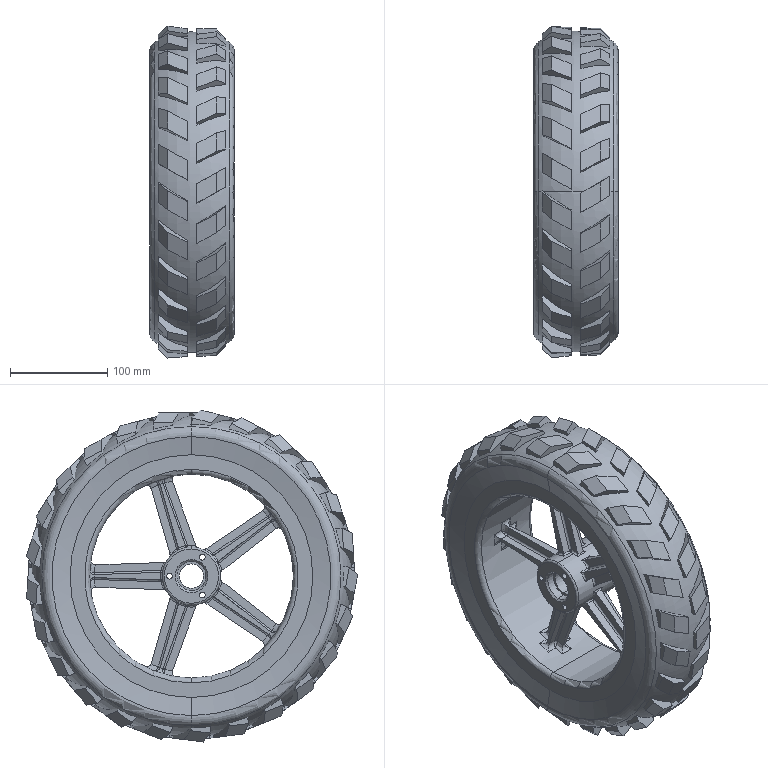Part | SolidWorks | features CirPattern 5, ICE 5, Fillet 3, Chamfer 2, Revolution 2 | 1 solid | 654 faces | box 87.248 x 341.454 x 341.945 mm | volume 1756971 mm3 | plane 368 | cylinder 120 | spline 110 | torus 24 | sphere 20 | cone 12 | commonest cylinder face diameters 4 x55 10 x39 6 x6 30 x4 260 x4 25 x2